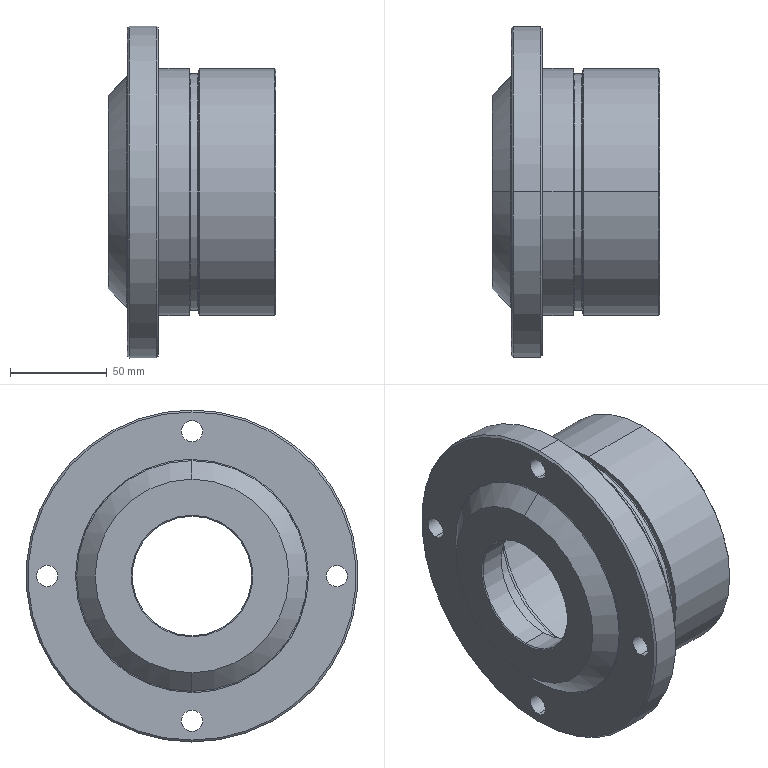Part | SolidWorks | features BaseBody 1 | 1 solid | 71 faces | box 86.84 x 172 x 172 mm | volume 557963 mm3 | cylinder 28 | spline 18 | cone 16 | plane 9 | commonest cylinder face diameters 11 x8 110 x4 128 x4 62 x2 90 x2 100 x2